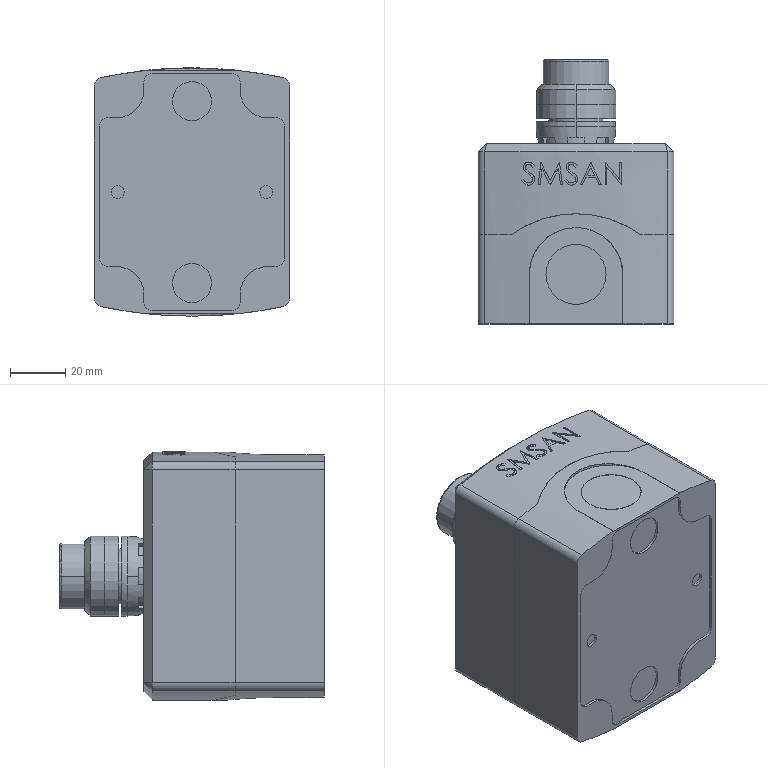Part | NX | features BREP 14 | 14 solids | 1183 faces | box 71 x 96 x 90.1 mm | volume 166957 mm3 | plane 594 | cylinder 373 | torus 68 | spline 68 | sphere 63 | cone 17 | commonest cylinder face diameters 0.2 x176 0.4 x20 2 x18 6 x18 25 x16 20 x11